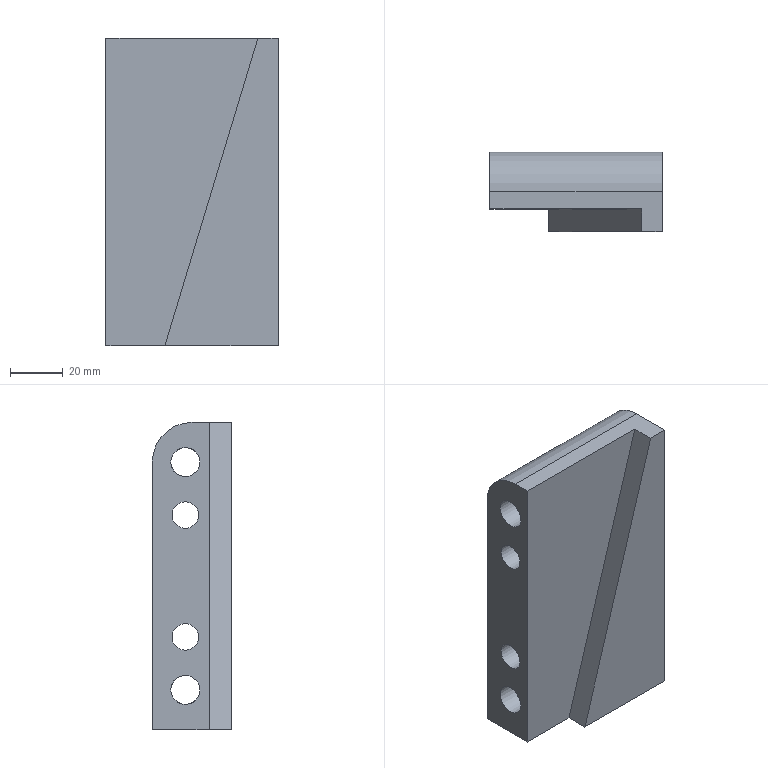Part | STEP file | solid 241 | 1 solid | 17 faces | box 65 x 30 x 116 mm | volume 157735 mm3 | plane 10 | cylinder 7 | commonest cylinder face diameters 10 x2 11 x2 18 x2 30 x1